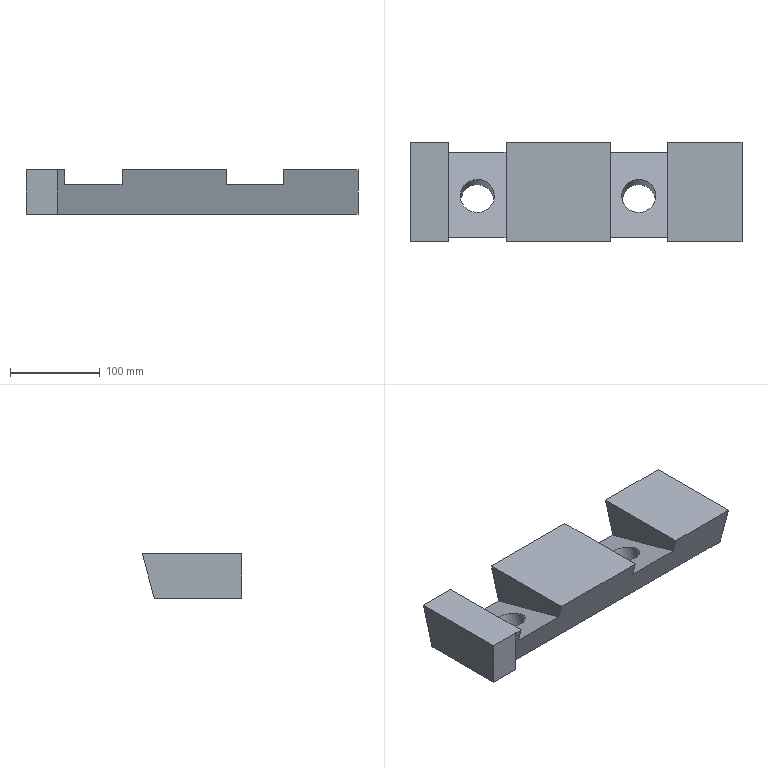Part | SolidWorks | features ICE 3, Extrusion 1, LPattern 1, RevCut 1 | 1 solid | 20 faces | box 370 x 110.795 x 50 mm | volume 1371734 mm3 | plane 16 | cylinder 4 | commonest cylinder face diameters 38 x4
STEP:
#1=CARTESIAN_POINT('',(70.,69.461,-33.943));
#2=VERTEX_POINT('',#1);
#3=CARTESIAN_POINT('',(70.,32.616,-24.071));
#4=VERTEX_POINT('',#3);
#5=CARTESIAN_POINT('',(70.,69.461,-33.943));
#6=CARTESIAN_POINT('',(32.,69.461,-33.943));
#7=CARTESIAN_POINT('',(32.,32.616,-24.071));
#8=CARTESIAN_POINT('',(70.,32.616,-24.071));
#9=(BOUNDED_CURVE()B_SPLINE_CURVE(3,(#5,#6,#7,#8),.UNSPECIFIED.,.F.,.F.)B_SPLINE_CURVE_WITH_KNOTS((4,4),(3.142,6.283),.UNSPECIFIED.)CURVE()GEOMETRIC_REPRESENTATION_ITEM()RATIONAL_B_SPLINE_CURVE((1.,0.3333,0.3333,1.))REPRESENTATION_ITEM(''));
#10=EDGE_CURVE('',#2,#4,#9,.T.);
#11=ORIENTED_EDGE('',*,*,#10,.T.);
#12=CARTESIAN_POINT('',(70.,23.178,-50.));
#13=VERTEX_POINT('',#12);
#14=CARTESIAN_POINT('',(70.,13.311,-77.108));
#15=DIRECTION('',(0.,-0.342,-0.9397));
#16=VECTOR('',#15,1000.);
#17=LINE('',#14,#16);
#18=EDGE_CURVE('',#4,#13,#17,.T.);
#19=ORIENTED_EDGE('',*,*,#18,.T.);
#20=CARTESIAN_POINT('',(70.,63.617,-50.));
#21=VERTEX_POINT('',#20);
#22=CARTESIAN_POINT('',(70.,23.178,-50.));
#23=CARTESIAN_POINT('',(32.,23.178,-50.));
#24=CARTESIAN_POINT('',(32.,63.617,-50.));
#25=CARTESIAN_POINT('',(70.,63.617,-50.));
#26=(BOUNDED_CURVE()B_SPLINE_CURVE(3,(#22,#23,#24,#25),.UNSPECIFIED.,.F.,.F.)B_SPLINE_CURVE_WITH_KNOTS((4,4),(0.,3.142),.UNSPECIFIED.)CURVE()GEOMETRIC_REPRESENTATION_ITEM()RATIONAL_B_SPLINE_CURVE((1.,0.3333,0.3333,1.))REPRESENTATION_ITEM(''));
#27=EDGE_CURVE('',#13,#21,#26,.T.);
#28=ORIENTED_EDGE('',*,*,#27,.T.);
#29=CARTESIAN_POINT('',(70.,49.02,-90.105));
#30=DIRECTION('',(0.,-0.342,-0.9397));
#31=VECTOR('',#30,1000.);
#32=LINE('',#29,#31);
#33=EDGE_CURVE('',#2,#21,#32,.T.);
#34=ORIENTED_EDGE('',*,*,#33,.F.);
#35=EDGE_LOOP('',(#11,#19,#28,#34));
#36=FACE_OUTER_BOUND('',#35,.T.);
#37=CARTESIAN_POINT('',(70.,31.166,-83.607));
#38=DIRECTION('',(0.,-0.342,-0.9397));
#39=DIRECTION('',(0.,0.9397,-0.342));
#40=AXIS2_PLACEMENT_3D('',#37,#38,#39);
#41=CYLINDRICAL_SURFACE('',#40,19.);
#42=ADVANCED_FACE('',(#36),#41,.F.);
#43=CARTESIAN_POINT('',(-110.,69.461,-33.943));
#44=VERTEX_POINT('',#43);
#45=CARTESIAN_POINT('',(-110.,32.616,-24.071));
#46=VERTEX_POINT('',#45);
#47=CARTESIAN_POINT('',(-110.,69.461,-33.943));
#48=CARTESIAN_POINT('',(-148.,69.461,-33.943));
#49=CARTESIAN_POINT('',(-148.,32.616,-24.071));
#50=CARTESIAN_POINT('',(-110.,32.616,-24.071));
#51=(BOUNDED_CURVE()B_SPLINE_CURVE(3,(#47,#48,#49,#50),.UNSPECIFIED.,.F.,.F.)B_SPLINE_CURVE_WITH_KNOTS((4,4),(3.142,6.283),.UNSPECIFIED.)CURVE()GEOMETRIC_REPRESENTATION_ITEM()RATIONAL_B_SPLINE_CURVE((1.,0.3333,0.3333,1.))REPRESENTATION_ITEM(''));
#52=EDGE_CURVE('',#44,#46,#51,.T.);
#53=ORIENTED_EDGE('',*,*,#52,.T.);
#54=CARTESIAN_POINT('',(-110.,23.178,-50.));
#55=VERTEX_POINT('',#54);
#56=CARTESIAN_POINT('',(-110.,13.311,-77.108));
#57=DIRECTION('',(0.,-0.342,-0.9397));
#58=VECTOR('',#57,1000.);
#59=LINE('',#56,#58);
#60=EDGE_CURVE('',#46,#55,#59,.T.);
#61=ORIENTED_EDGE('',*,*,#60,.T.);
#62=CARTESIAN_POINT('',(-110.,63.617,-50.));
#63=VERTEX_POINT('',#62);
#64=CARTESIAN_POINT('',(-110.,23.178,-50.));
#65=CARTESIAN_POINT('',(-148.,23.178,-50.));
#66=CARTESIAN_POINT('',(-148.,63.617,-50.));
#67=CARTESIAN_POINT('',(-110.,63.617,-50.));
#68=(BOUNDED_CURVE()B_SPLINE_CURVE(3,(#64,#65,#66,#67),.UNSPECIFIED.,.F.,.F.)B_SPLINE_CURVE_WITH_KNOTS((4,4),(0.,3.142),.UNSPECIFIED.)CURVE()GEOMETRIC_REPRESENTATION_ITEM()RATIONAL_B_SPLINE_CURVE((1.,0.3333,0.3333,1.))REPRESENTATION_ITEM(''));
#69=EDGE_CURVE('',#55,#63,#68,.T.);
#70=ORIENTED_EDGE('',*,*,#69,.T.);
#71=CARTESIAN_POINT('',(-110.,49.02,-90.105));
#72=DIRECTION('',(0.,-0.342,-0.9397));
#73=VECTOR('',#72,1000.);
#74=LINE('',#71,#73);
#75=EDGE_CURVE('',#44,#63,#74,.T.);
#76=ORIENTED_EDGE('',*,*,#75,.F.);
#77=EDGE_LOOP('',(#53,#61,#70,#76));
#78=FACE_OUTER_BOUND('',#77,.T.);
#79=CARTESIAN_POINT('',(-110.,31.166,-83.607));
#80=DIRECTION('',(0.,-0.342,-0.9397));
#81=DIRECTION('',(0.,0.9397,-0.342));
#82=AXIS2_PLACEMENT_3D('',#79,#80,#81);
#83=CYLINDRICAL_SURFACE('',#82,19.);
#84=ADVANCED_FACE('',(#78),#83,.F.);
#85=CARTESIAN_POINT('',(102.,110.795,0.));
#86=VERTEX_POINT('',#85);
#87=CARTESIAN_POINT('',(102.,0.,0.));
#88=VERTEX_POINT('',#87);
#89=CARTESIAN_POINT('',(102.,110.795,0.));
#90=DIRECTION('',(0.,-1.,0.));
#91=VECTOR('',#90,1000.);
#92=LINE('',#89,#91);
#93=EDGE_CURVE('',#86,#88,#92,.T.);
#94=ORIENTED_EDGE('',*,*,#93,.T.);
#95=CARTESIAN_POINT('',(185.,0.,0.));
#96=VERTEX_POINT('',#95);
#97=CARTESIAN_POINT('',(185.,0.,0.));
#98=DIRECTION('',(-1.,0.,0.));
#99=VECTOR('',#98,1000.);
#100=LINE('',#97,#99);
#101=EDGE_CURVE('',#96,#88,#100,.T.);
#102=ORIENTED_EDGE('',*,*,#101,.F.);
#103=CARTESIAN_POINT('',(185.,110.795,0.));
#104=VERTEX_POINT('',#103);
#105=CARTESIAN_POINT('',(185.,0.,0.));
#106=DIRECTION('',(0.,-1.,0.));
#107=VECTOR('',#106,1000.);
#108=LINE('',#105,#107);
#109=EDGE_CURVE('',#104,#96,#108,.T.);
#110=ORIENTED_EDGE('',*,*,#109,.F.);
#111=CARTESIAN_POINT('',(185.,110.795,0.));
#112=DIRECTION('',(-1.,0.,0.));
#113=VECTOR('',#112,1000.);
#114=LINE('',#111,#113);
#115=EDGE_CURVE('',#104,#86,#114,.T.);
#116=ORIENTED_EDGE('',*,*,#115,.T.);
#117=EDGE_LOOP('',(#94,#102,#110,#116));
#118=FACE_OUTER_BOUND('',#117,.T.);
#119=CARTESIAN_POINT('',(185.,0.,0.));
#120=DIRECTION('',(0.,0.,-1.));
#121=DIRECTION('',(0.,1.,0.));
#122=AXIS2_PLACEMENT_3D('',#119,#120,#121);
#123=PLANE('',#122);
#124=ADVANCED_FACE('',(#118),#123,.F.);
#125=CARTESIAN_POINT('',(38.,0.,0.));
#126=VERTEX_POINT('',#125);
#127=CARTESIAN_POINT('',(-78.,0.,0.));
#128=VERTEX_POINT('',#127);
#129=CARTESIAN_POINT('',(185.,0.,0.));
#130=DIRECTION('',(-1.,0.,0.));
#131=VECTOR('',#130,1000.);
#132=LINE('',#129,#131);
#133=EDGE_CURVE('',#126,#128,#132,.T.);
#134=ORIENTED_EDGE('',*,*,#133,.F.);
#135=CARTESIAN_POINT('',(38.,110.795,0.));
#136=VERTEX_POINT('',#135);
#137=CARTESIAN_POINT('',(38.,110.795,0.));
#138=DIRECTION('',(0.,-1.,0.));
#139=VECTOR('',#138,1000.);
#140=LINE('',#137,#139);
#141=EDGE_CURVE('',#136,#126,#140,.T.);
#142=ORIENTED_EDGE('',*,*,#141,.F.);
#143=CARTESIAN_POINT('',(-78.,110.795,0.));
#144=VERTEX_POINT('',#143);
#145=CARTESIAN_POINT('',(185.,110.795,0.));
#146=DIRECTION('',(-1.,0.,0.));
#147=VECTOR('',#146,1000.);
#148=LINE('',#145,#147);
#149=EDGE_CURVE('',#136,#144,#148,.T.);
#150=ORIENTED_EDGE('',*,*,#149,.T.);
#151=CARTESIAN_POINT('',(-78.,110.795,0.));
#152=DIRECTION('',(0.,-1.,0.));
#153=VECTOR('',#152,1000.);
#154=LINE('',#151,#153);
#155=EDGE_CURVE('',#144,#128,#154,.T.);
#156=ORIENTED_EDGE('',*,*,#155,.T.);
#157=EDGE_LOOP('',(#134,#142,#150,#156));
#158=FACE_OUTER_BOUND('',#157,.T.);
#159=CARTESIAN_POINT('',(185.,0.,0.));
#160=DIRECTION('',(0.,0.,-1.));
#161=DIRECTION('',(0.,1.,0.));
#162=AXIS2_PLACEMENT_3D('',#159,#160,#161);
#163=PLANE('',#162);
#164=ADVANCED_FACE('',(#158),#163,.F.);
#165=CARTESIAN_POINT('',(38.,4.426,-16.517));
#166=VERTEX_POINT('',#165);
#167=CARTESIAN_POINT('',(102.,4.426,-16.517));
#168=VERTEX_POINT('',#167);
#169=CARTESIAN_POINT('',(38.,4.426,-16.517));
#170=DIRECTION('',(1.,0.,0.));
#171=VECTOR('',#170,1000.);
#172=LINE('',#169,#171);
#173=EDGE_CURVE('',#166,#168,#172,.T.);
#174=ORIENTED_EDGE('',*,*,#173,.F.);
#175=CARTESIAN_POINT('',(38.,0.,0.));
#176=DIRECTION('',(0.,0.2588,-0.9659));
#177=VECTOR('',#176,1000.);
#178=LINE('',#175,#177);
#179=EDGE_CURVE('',#126,#166,#178,.T.);
#180=ORIENTED_EDGE('',*,*,#179,.F.);
#181=ORIENTED_EDGE('',*,*,#133,.T.);
#182=CARTESIAN_POINT('',(-78.,4.426,-16.517));
#183=VERTEX_POINT('',#182);
#184=CARTESIAN_POINT('',(-78.,0.,0.));
#185=DIRECTION('',(0.,0.2588,-0.9659));
#186=VECTOR('',#185,1000.);
#187=LINE('',#184,#186);
#188=EDGE_CURVE('',#128,#183,#187,.T.);
#189=ORIENTED_EDGE('',*,*,#188,.T.);
#190=CARTESIAN_POINT('',(-142.,4.426,-16.517));
#191=VERTEX_POINT('',#190);
#192=CARTESIAN_POINT('',(-142.,4.426,-16.517));
#193=DIRECTION('',(1.,0.,0.));
#194=VECTOR('',#193,1000.);
#195=LINE('',#192,#194);
#196=EDGE_CURVE('',#191,#183,#195,.T.);
#197=ORIENTED_EDGE('',*,*,#196,.F.);
#198=CARTESIAN_POINT('',(-142.,0.,0.));
#199=VERTEX_POINT('',#198);
#200=CARTESIAN_POINT('',(-142.,0.,0.));
#201=DIRECTION('',(0.,0.2588,-0.9659));
#202=VECTOR('',#201,1000.);
#203=LINE('',#200,#202);
#204=EDGE_CURVE('',#199,#191,#203,.T.);
#205=ORIENTED_EDGE('',*,*,#204,.F.);
#206=CARTESIAN_POINT('',(-150.,0.,0.));
#207=VERTEX_POINT('',#206);
#208=CARTESIAN_POINT('',(185.,0.,0.));
#209=DIRECTION('',(-1.,0.,0.));
#210=VECTOR('',#209,1000.);
#211=LINE('',#208,#210);
#212=EDGE_CURVE('',#199,#207,#211,.T.);
#213=ORIENTED_EDGE('',*,*,#212,.T.);
#214=CARTESIAN_POINT('',(-150.,13.397,-50.));
#215=VERTEX_POINT('',#214);
#216=CARTESIAN_POINT('',(-150.,13.397,-50.));
#217=DIRECTION('',(0.,0.2588,-0.9659));
#218=VECTOR('',#217,1000.);
#219=LINE('',#216,#218);
#220=EDGE_CURVE('',#207,#215,#219,.T.);
#221=ORIENTED_EDGE('',*,*,#220,.T.);
#222=CARTESIAN_POINT('',(185.,13.397,-50.));
#223=VERTEX_POINT('',#222);
#224=CARTESIAN_POINT('',(185.,13.397,-50.));
#225=DIRECTION('',(-1.,0.,0.));
#226=VECTOR('',#225,1000.);
#227=LINE('',#224,#226);
#228=EDGE_CURVE('',#223,#215,#227,.T.);
#229=ORIENTED_EDGE('',*,*,#228,.F.);
#230=CARTESIAN_POINT('',(185.,13.397,-50.));
#231=DIRECTION('',(0.,0.2588,-0.9659));
#232=VECTOR('',#231,1000.);
#233=LINE('',#230,#232);
#234=EDGE_CURVE('',#96,#223,#233,.T.);
#235=ORIENTED_EDGE('',*,*,#234,.F.);
#236=ORIENTED_EDGE('',*,*,#101,.T.);
#237=CARTESIAN_POINT('',(102.,0.,0.));
#238=DIRECTION('',(0.,0.2588,-0.9659));
#239=VECTOR('',#238,1000.);
#240=LINE('',#237,#239);
#241=EDGE_CURVE('',#88,#168,#240,.T.);
#242=ORIENTED_EDGE('',*,*,#241,.T.);
#243=EDGE_LOOP('',(#174,#180,#181,#189,#197,#205,#213,#221,#229,#235,#236,#242));
#244=FACE_OUTER_BOUND('',#243,.T.);
#245=CARTESIAN_POINT('',(185.,13.397,-50.));
#246=DIRECTION('',(0.,0.9659,0.2588));
#247=DIRECTION('',(0.,-0.2588,0.9659));
#248=AXIS2_PLACEMENT_3D('',#245,#246,#247);
#249=PLANE('',#248);
#250=ADVANCED_FACE('',(#244),#249,.F.);
#251=CARTESIAN_POINT('',(70.,63.617,-50.));
#252=CARTESIAN_POINT('',(108.,63.617,-50.));
#253=CARTESIAN_POINT('',(108.,23.178,-50.));
#254=CARTESIAN_POINT('',(70.,23.178,-50.));
#255=(BOUNDED_CURVE()B_SPLINE_CURVE(3,(#251,#252,#253,#254),.UNSPECIFIED.,.F.,.T.)B_SPLINE_CURVE_WITH_KNOTS((4,4),(3.142,6.283),.UNSPECIFIED.)CURVE()GEOMETRIC_REPRESENTATION_ITEM()RATIONAL_B_SPLINE_CURVE((1.,0.3333,0.3333,1.))REPRESENTATION_ITEM(''));
#256=EDGE_CURVE('',#21,#13,#255,.T.);
#257=ORIENTED_EDGE('',*,*,#256,.F.);
#258=ORIENTED_EDGE('',*,*,#27,.F.);
#259=EDGE_LOOP('',(#257,#258));
#260=FACE_BOUND('',#259,.T.);
#261=CARTESIAN_POINT('',(-110.,63.617,-50.));
#262=CARTESIAN_POINT('',(-72.,63.617,-50.));
#263=CARTESIAN_POINT('',(-72.,23.178,-50.));
#264=CARTESIAN_POINT('',(-110.,23.178,-50.));
#265=(BOUNDED_CURVE()B_SPLINE_CURVE(3,(#261,#262,#263,#264),.UNSPECIFIED.,.F.,.T.)B_SPLINE_CURVE_WITH_KNOTS((4,4),(3.142,6.283),.UNSPECIFIED.)CURVE()GEOMETRIC_REPRESENTATION_ITEM()RATIONAL_B_SPLINE_CURVE((1.,0.3333,0.3333,1.))REPRESENTATION_ITEM(''));
#266=EDGE_CURVE('',#63,#55,#265,.T.);
#267=ORIENTED_EDGE('',*,*,#266,.F.);
#268=ORIENTED_EDGE('',*,*,#69,.F.);
#269=EDGE_LOOP('',(#267,#268));
#270=FACE_BOUND('',#269,.T.);
#271=CARTESIAN_POINT('',(-185.,0.,-50.));
#272=VERTEX_POINT('',#271);
#273=CARTESIAN_POINT('',(-185.,97.397,-50.));
#274=VERTEX_POINT('',#273);
#275=CARTESIAN_POINT('',(-185.,97.397,-50.));
#276=DIRECTION('',(0.,1.,0.));
#277=VECTOR('',#276,1000.);
#278=LINE('',#275,#277);
#279=EDGE_CURVE('',#272,#274,#278,.T.);
#280=ORIENTED_EDGE('',*,*,#279,.T.);
#281=CARTESIAN_POINT('',(185.,97.397,-50.));
#282=VERTEX_POINT('',#281);
#283=CARTESIAN_POINT('',(185.,97.397,-50.));
#284=DIRECTION('',(-1.,0.,0.));
#285=VECTOR('',#284,1000.);
#286=LINE('',#283,#285);
#287=EDGE_CURVE('',#282,#274,#286,.T.);
#288=ORIENTED_EDGE('',*,*,#287,.F.);
#289=CARTESIAN_POINT('',(185.,97.397,-50.));
#290=DIRECTION('',(0.,1.,0.));
#291=VECTOR('',#290,1000.);
#292=LINE('',#289,#291);
#293=EDGE_CURVE('',#223,#282,#292,.T.);
#294=ORIENTED_EDGE('',*,*,#293,.F.);
#295=ORIENTED_EDGE('',*,*,#228,.T.);
#296=CARTESIAN_POINT('',(-150.,0.,-50.));
#297=VERTEX_POINT('',#296);
#298=CARTESIAN_POINT('',(-150.,0.,-50.));
#299=DIRECTION('',(0.,-1.,0.));
#300=VECTOR('',#299,1000.);
#301=LINE('',#298,#300);
#302=EDGE_CURVE('',#215,#297,#301,.T.);
#303=ORIENTED_EDGE('',*,*,#302,.T.);
#304=CARTESIAN_POINT('',(-150.,0.,-50.));
#305=DIRECTION('',(-1.,0.,0.));
#306=VECTOR('',#305,1000.);
#307=LINE('',#304,#306);
#308=EDGE_CURVE('',#297,#272,#307,.T.);
#309=ORIENTED_EDGE('',*,*,#308,.T.);
#310=EDGE_LOOP('',(#280,#288,#294,#295,#303,#309));
#311=FACE_OUTER_BOUND('',#310,.T.);
#312=CARTESIAN_POINT('',(185.,97.397,-50.));
#313=DIRECTION('',(0.,0.,1.));
#314=DIRECTION('',(0.,-1.,0.));
#315=AXIS2_PLACEMENT_3D('',#312,#313,#314);
#316=PLANE('',#315);
#317=ADVANCED_FACE('',(#260,#270,#311),#316,.F.);
#318=ORIENTED_EDGE('',*,*,#149,.F.);
#319=CARTESIAN_POINT('',(38.,99.54,-42.003));
#320=VERTEX_POINT('',#319);
#321=CARTESIAN_POINT('',(38.,99.54,-42.003));
#322=DIRECTION('',(0.,0.2588,0.9659));
#323=VECTOR('',#322,1000.);
#324=LINE('',#321,#323);
#325=EDGE_CURVE('',#320,#136,#324,.T.);
#326=ORIENTED_EDGE('',*,*,#325,.F.);
#327=CARTESIAN_POINT('',(102.,99.54,-42.003));
#328=VERTEX_POINT('',#327);
#329=CARTESIAN_POINT('',(38.,99.54,-42.003));
#330=DIRECTION('',(1.,0.,0.));
#331=VECTOR('',#330,1000.);
#332=LINE('',#329,#331);
#333=EDGE_CURVE('',#320,#328,#332,.T.);
#334=ORIENTED_EDGE('',*,*,#333,.T.);
#335=CARTESIAN_POINT('',(102.,99.54,-42.003));
#336=DIRECTION('',(0.,0.2588,0.9659));
#337=VECTOR('',#336,1000.);
#338=LINE('',#335,#337);
#339=EDGE_CURVE('',#328,#86,#338,.T.);
#340=ORIENTED_EDGE('',*,*,#339,.T.);
#341=ORIENTED_EDGE('',*,*,#115,.F.);
#342=CARTESIAN_POINT('',(185.,110.795,0.));
#343=DIRECTION('',(0.,0.2588,0.9659));
#344=VECTOR('',#343,1000.);
#345=LINE('',#342,#344);
#346=EDGE_CURVE('',#282,#104,#345,.T.);
#347=ORIENTED_EDGE('',*,*,#346,.F.);
#348=ORIENTED_EDGE('',*,*,#287,.T.);
#349=CARTESIAN_POINT('',(-185.,110.795,0.));
#350=VERTEX_POINT('',#349);
#351=CARTESIAN_POINT('',(-185.,110.795,0.));
#352=DIRECTION('',(0.,0.2588,0.9659));
#353=VECTOR('',#352,1000.);
#354=LINE('',#351,#353);
#355=EDGE_CURVE('',#274,#350,#354,.T.);
#356=ORIENTED_EDGE('',*,*,#355,.T.);
#357=CARTESIAN_POINT('',(-142.,110.795,0.));
#358=VERTEX_POINT('',#357);
#359=CARTESIAN_POINT('',(185.,110.795,0.));
#360=DIRECTION('',(-1.,0.,0.));
#361=VECTOR('',#360,1000.);
#362=LINE('',#359,#361);
#363=EDGE_CURVE('',#358,#350,#362,.T.);
#364=ORIENTED_EDGE('',*,*,#363,.F.);
#365=CARTESIAN_POINT('',(-142.,99.54,-42.003));
#366=VERTEX_POINT('',#365);
#367=CARTESIAN_POINT('',(-142.,99.54,-42.003));
#368=DIRECTION('',(0.,0.2588,0.9659));
#369=VECTOR('',#368,1000.);
#370=LINE('',#367,#369);
#371=EDGE_CURVE('',#366,#358,#370,.T.);
#372=ORIENTED_EDGE('',*,*,#371,.F.);
#373=CARTESIAN_POINT('',(-78.,99.54,-42.003));
#374=VERTEX_POINT('',#373);
#375=CARTESIAN_POINT('',(-142.,99.54,-42.003));
#376=DIRECTION('',(1.,0.,0.));
#377=VECTOR('',#376,1000.);
#378=LINE('',#375,#377);
#379=EDGE_CURVE('',#366,#374,#378,.T.);
#380=ORIENTED_EDGE('',*,*,#379,.T.);
#381=CARTESIAN_POINT('',(-78.,99.54,-42.003));
#382=DIRECTION('',(0.,0.2588,0.9659));
#383=VECTOR('',#382,1000.);
#384=LINE('',#381,#383);
#385=EDGE_CURVE('',#374,#144,#384,.T.);
#386=ORIENTED_EDGE('',*,*,#385,.T.);
#387=EDGE_LOOP('',(#318,#326,#334,#340,#341,#347,#348,#356,#364,#372,#380,#386));
#388=FACE_OUTER_BOUND('',#387,.T.);
#389=CARTESIAN_POINT('',(185.,110.795,0.));
#390=DIRECTION('',(0.,-0.9659,0.2588));
#391=DIRECTION('',(0.,-0.2588,-0.9659));
#392=AXIS2_PLACEMENT_3D('',#389,#390,#391);
#393=PLANE('',#392);
#394=ADVANCED_FACE('',(#388),#393,.F.);
#395=ORIENTED_EDGE('',*,*,#212,.F.);
#396=CARTESIAN_POINT('',(-142.,110.795,0.));
#397=DIRECTION('',(0.,-1.,0.));
#398=VECTOR('',#397,1000.);
#399=LINE('',#396,#398);
#400=EDGE_CURVE('',#358,#199,#399,.T.);
#401=ORIENTED_EDGE('',*,*,#400,.F.);
#402=ORIENTED_EDGE('',*,*,#363,.T.);
#403=CARTESIAN_POINT('',(-185.,0.,0.));
#404=VERTEX_POINT('',#403);
#405=CARTESIAN_POINT('',(-185.,0.,0.));
#406=DIRECTION('',(0.,-1.,0.));
#407=VECTOR('',#406,1000.);
#408=LINE('',#405,#407);
#409=EDGE_CURVE('',#350,#404,#408,.T.);
#410=ORIENTED_EDGE('',*,*,#409,.T.);
#411=CARTESIAN_POINT('',(-150.,0.,0.));
#412=DIRECTION('',(-1.,0.,0.));
#413=VECTOR('',#412,1000.);
#414=LINE('',#411,#413);
#415=EDGE_CURVE('',#207,#404,#414,.T.);
#416=ORIENTED_EDGE('',*,*,#415,.F.);
#417=EDGE_LOOP('',(#395,#401,#402,#410,#416));
#418=FACE_OUTER_BOUND('',#417,.T.);
#419=CARTESIAN_POINT('',(185.,0.,0.));
#420=DIRECTION('',(0.,0.,-1.));
#421=DIRECTION('',(0.,1.,0.));
#422=AXIS2_PLACEMENT_3D('',#419,#420,#421);
#423=PLANE('',#422);
#424=ADVANCED_FACE('',(#418),#423,.F.);
#425=ORIENTED_EDGE('',*,*,#234,.T.);
#426=ORIENTED_EDGE('',*,*,#293,.T.);
#427=ORIENTED_EDGE('',*,*,#346,.T.);
#428=ORIENTED_EDGE('',*,*,#109,.T.);
#429=EDGE_LOOP('',(#425,#426,#427,#428));
#430=FACE_OUTER_BOUND('',#429,.T.);
#431=CARTESIAN_POINT('',(185.,0.,0.));
#432=DIRECTION('',(-1.,0.,0.));
#433=DIRECTION('',(0.,0.,1.));
#434=AXIS2_PLACEMENT_3D('',#431,#432,#433);
#435=PLANE('',#434);
#436=ADVANCED_FACE('',(#430),#435,.F.);
#437=ORIENTED_EDGE('',*,*,#279,.F.);
#438=CARTESIAN_POINT('',(-185.,0.,0.));
#439=DIRECTION('',(0.,0.,1.));
#440=VECTOR('',#439,1000.);
#441=LINE('',#438,#440);
#442=EDGE_CURVE('',#272,#404,#441,.T.);
#443=ORIENTED_EDGE('',*,*,#442,.T.);
#444=ORIENTED_EDGE('',*,*,#409,.F.);
#445=ORIENTED_EDGE('',*,*,#355,.F.);
#446=EDGE_LOOP('',(#437,#443,#444,#445));
#447=FACE_OUTER_BOUND('',#446,.T.);
#448=CARTESIAN_POINT('',(-185.,0.,0.));
#449=DIRECTION('',(-1.,0.,0.));
#450=DIRECTION('',(0.,0.,1.));
#451=AXIS2_PLACEMENT_3D('',#448,#449,#450);
#452=PLANE('',#451);
#453=ADVANCED_FACE('',(#447),#452,.T.);
#454=ORIENTED_EDGE('',*,*,#442,.F.);
#455=ORIENTED_EDGE('',*,*,#308,.F.);
#456=CARTESIAN_POINT('',(-150.,0.,0.));
#457=DIRECTION('',(0.,0.,1.));
#458=VECTOR('',#457,1000.);
#459=LINE('',#456,#458);
#460=EDGE_CURVE('',#297,#207,#459,.T.);
#461=ORIENTED_EDGE('',*,*,#460,.T.);
#462=ORIENTED_EDGE('',*,*,#415,.T.);
#463=EDGE_LOOP('',(#454,#455,#461,#462));
#464=FACE_OUTER_BOUND('',#463,.T.);
#465=CARTESIAN_POINT('',(-150.,0.,0.));
#466=DIRECTION('',(0.,-1.,0.));
#467=DIRECTION('',(0.,0.,-1.));
#468=AXIS2_PLACEMENT_3D('',#465,#466,#467);
#469=PLANE('',#468);
#470=ADVANCED_FACE('',(#464),#469,.T.);
#471=ORIENTED_EDGE('',*,*,#220,.F.);
#472=ORIENTED_EDGE('',*,*,#460,.F.);
#473=ORIENTED_EDGE('',*,*,#302,.F.);
#474=EDGE_LOOP('',(#471,#472,#473));
#475=FACE_OUTER_BOUND('',#474,.T.);
#476=CARTESIAN_POINT('',(-150.,0.,0.));
#477=DIRECTION('',(-1.,0.,0.));
#478=DIRECTION('',(0.,0.,1.));
#479=AXIS2_PLACEMENT_3D('',#476,#477,#478);
#480=PLANE('',#479);
#481=ADVANCED_FACE('',(#475),#480,.F.);
#482=ORIENTED_EDGE('',*,*,#52,.F.);
#483=CARTESIAN_POINT('',(-110.,32.616,-24.071));
#484=CARTESIAN_POINT('',(-72.,32.616,-24.071));
#485=CARTESIAN_POINT('',(-72.,69.461,-33.943));
#486=CARTESIAN_POINT('',(-110.,69.461,-33.943));
#487=(BOUNDED_CURVE()B_SPLINE_CURVE(3,(#483,#484,#485,#486),.UNSPECIFIED.,.F.,.F.)B_SPLINE_CURVE_WITH_KNOTS((4,4),(0.,3.142),.UNSPECIFIED.)CURVE()GEOMETRIC_REPRESENTATION_ITEM()RATIONAL_B_SPLINE_CURVE((1.,0.3333,0.3333,1.))REPRESENTATION_ITEM(''));
#488=EDGE_CURVE('',#46,#44,#487,.T.);
#489=ORIENTED_EDGE('',*,*,#488,.F.);
#490=EDGE_LOOP('',(#482,#489));
#491=FACE_BOUND('',#490,.T.);
#492=CARTESIAN_POINT('',(-78.,4.426,-16.517));
#493=DIRECTION('',(0.,0.9659,-0.2588));
#494=VECTOR('',#493,1000.);
#495=LINE('',#492,#494);
#496=EDGE_CURVE('',#183,#374,#495,.T.);
#497=ORIENTED_EDGE('',*,*,#496,.T.);
#498=ORIENTED_EDGE('',*,*,#379,.F.);
#499=CARTESIAN_POINT('',(-142.,4.426,-16.517));
#500=DIRECTION('',(0.,0.9659,-0.2588));
#501=VECTOR('',#500,1000.);
#502=LINE('',#499,#501);
#503=EDGE_CURVE('',#191,#366,#502,.T.);
#504=ORIENTED_EDGE('',*,*,#503,.F.);
#505=ORIENTED_EDGE('',*,*,#196,.T.);
#506=EDGE_LOOP('',(#497,#498,#504,#505));
#507=FACE_OUTER_BOUND('',#506,.T.);
#508=CARTESIAN_POINT('',(-142.,4.426,-16.517));
#509=DIRECTION('',(0.,-0.2588,-0.9659));
#510=DIRECTION('',(0.,0.9659,-0.2588));
#511=AXIS2_PLACEMENT_3D('',#508,#509,#510);
#512=PLANE('',#511);
#513=ADVANCED_FACE('',(#491,#507),#512,.F.);
#514=ORIENTED_EDGE('',*,*,#204,.T.);
#515=ORIENTED_EDGE('',*,*,#503,.T.);
#516=ORIENTED_EDGE('',*,*,#371,.T.);
#517=ORIENTED_EDGE('',*,*,#400,.T.);
#518=EDGE_LOOP('',(#514,#515,#516,#517));
#519=FACE_OUTER_BOUND('',#518,.T.);
#520=CARTESIAN_POINT('',(-142.,0.,0.));
#521=DIRECTION('',(-1.,0.,0.));
#522=DIRECTION('',(0.,0.,1.));
#523=AXIS2_PLACEMENT_3D('',#520,#521,#522);
#524=PLANE('',#523);
#525=ADVANCED_FACE('',(#519),#524,.F.);
#526=ORIENTED_EDGE('',*,*,#188,.F.);
#527=ORIENTED_EDGE('',*,*,#155,.F.);
#528=ORIENTED_EDGE('',*,*,#385,.F.);
#529=ORIENTED_EDGE('',*,*,#496,.F.);
#530=EDGE_LOOP('',(#526,#527,#528,#529));
#531=FACE_OUTER_BOUND('',#530,.T.);
#532=CARTESIAN_POINT('',(-78.,0.,0.));
#533=DIRECTION('',(-1.,0.,0.));
#534=DIRECTION('',(0.,0.,1.));
#535=AXIS2_PLACEMENT_3D('',#532,#533,#534);
#536=PLANE('',#535);
#537=ADVANCED_FACE('',(#531),#536,.T.);
#538=ORIENTED_EDGE('',*,*,#10,.F.);
#539=CARTESIAN_POINT('',(70.,32.616,-24.071));
#540=CARTESIAN_POINT('',(108.,32.616,-24.071));
#541=CARTESIAN_POINT('',(108.,69.461,-33.943));
#542=CARTESIAN_POINT('',(70.,69.461,-33.943));
#543=(BOUNDED_CURVE()B_SPLINE_CURVE(3,(#539,#540,#541,#542),.UNSPECIFIED.,.F.,.F.)B_SPLINE_CURVE_WITH_KNOTS((4,4),(0.,3.142),.UNSPECIFIED.)CURVE()GEOMETRIC_REPRESENTATION_ITEM()RATIONAL_B_SPLINE_CURVE((1.,0.3333,0.3333,1.))REPRESENTATION_ITEM(''));
#544=EDGE_CURVE('',#4,#2,#543,.T.);
#545=ORIENTED_EDGE('',*,*,#544,.F.);
#546=EDGE_LOOP('',(#538,#545));
#547=FACE_BOUND('',#546,.T.);
#548=CARTESIAN_POINT('',(102.,4.426,-16.517));
#549=DIRECTION('',(0.,0.9659,-0.2588));
#550=VECTOR('',#549,1000.);
#551=LINE('',#548,#550);
#552=EDGE_CURVE('',#168,#328,#551,.T.);
#553=ORIENTED_EDGE('',*,*,#552,.T.);
#554=ORIENTED_EDGE('',*,*,#333,.F.);
#555=CARTESIAN_POINT('',(38.,4.426,-16.517));
#556=DIRECTION('',(0.,0.9659,-0.2588));
#557=VECTOR('',#556,1000.);
#558=LINE('',#555,#557);
#559=EDGE_CURVE('',#166,#320,#558,.T.);
#560=ORIENTED_EDGE('',*,*,#559,.F.);
#561=ORIENTED_EDGE('',*,*,#173,.T.);
#562=EDGE_LOOP('',(#553,#554,#560,#561));
#563=FACE_OUTER_BOUND('',#562,.T.);
#564=CARTESIAN_POINT('',(38.,4.426,-16.517));
#565=DIRECTION('',(0.,-0.2588,-0.9659));
#566=DIRECTION('',(0.,0.9659,-0.2588));
#567=AXIS2_PLACEMENT_3D('',#564,#565,#566);
#568=PLANE('',#567);
#569=ADVANCED_FACE('',(#547,#563),#568,.F.);
#570=ORIENTED_EDGE('',*,*,#179,.T.);
#571=ORIENTED_EDGE('',*,*,#559,.T.);
#572=ORIENTED_EDGE('',*,*,#325,.T.);
#573=ORIENTED_EDGE('',*,*,#141,.T.);
#574=EDGE_LOOP('',(#570,#571,#572,#573));
#575=FACE_OUTER_BOUND('',#574,.T.);
#576=CARTESIAN_POINT('',(38.,0.,0.));
#577=DIRECTION('',(-1.,0.,0.));
#578=DIRECTION('',(0.,0.,1.));
#579=AXIS2_PLACEMENT_3D('',#576,#577,#578);
#580=PLANE('',#579);
#581=ADVANCED_FACE('',(#575),#580,.F.);
#582=ORIENTED_EDGE('',*,*,#241,.F.);
#583=ORIENTED_EDGE('',*,*,#93,.F.);
#584=ORIENTED_EDGE('',*,*,#339,.F.);
#585=ORIENTED_EDGE('',*,*,#552,.F.);
#586=EDGE_LOOP('',(#582,#583,#584,#585));
#587=FACE_OUTER_BOUND('',#586,.T.);
#588=CARTESIAN_POINT('',(102.,0.,0.));
#589=DIRECTION('',(-1.,0.,0.));
#590=DIRECTION('',(0.,0.,1.));
#591=AXIS2_PLACEMENT_3D('',#588,#589,#590);
#592=PLANE('',#591);
#593=ADVANCED_FACE('',(#587),#592,.T.);
#594=ORIENTED_EDGE('',*,*,#60,.F.);
#595=ORIENTED_EDGE('',*,*,#488,.T.);
#596=ORIENTED_EDGE('',*,*,#75,.T.);
#597=ORIENTED_EDGE('',*,*,#266,.T.);
#598=EDGE_LOOP('',(#594,#595,#596,#597));
#599=FACE_OUTER_BOUND('',#598,.T.);
#600=CARTESIAN_POINT('',(-110.,31.166,-83.607));
#601=DIRECTION('',(0.,-0.342,-0.9397));
#602=DIRECTION('',(0.,0.9397,-0.342));
#603=AXIS2_PLACEMENT_3D('',#600,#601,#602);
#604=CYLINDRICAL_SURFACE('',#603,19.);
#605=ADVANCED_FACE('',(#599),#604,.F.);
#606=ORIENTED_EDGE('',*,*,#18,.F.);
#607=ORIENTED_EDGE('',*,*,#544,.T.);
#608=ORIENTED_EDGE('',*,*,#33,.T.);
#609=ORIENTED_EDGE('',*,*,#256,.T.);
#610=EDGE_LOOP('',(#606,#607,#608,#609));
#611=FACE_OUTER_BOUND('',#610,.T.);
#612=CARTESIAN_POINT('',(70.,31.166,-83.607));
#613=DIRECTION('',(0.,-0.342,-0.9397));
#614=DIRECTION('',(0.,0.9397,-0.342));
#615=AXIS2_PLACEMENT_3D('',#612,#613,#614);
#616=CYLINDRICAL_SURFACE('',#615,19.);
#617=ADVANCED_FACE('',(#611),#616,.F.);
#618=CLOSED_SHELL('',(#42,#84,#124,#164,#250,#317,#394,#424,#436,#453,#470,#481,#513,#525,#537,#569,#581,#593,#605,#617));
#619=MANIFOLD_SOLID_BREP('',#618);
#620=CARTESIAN_POINT('',(0.,0.,0.));
#621=DIRECTION('',(0.,0.,1.));
#622=DIRECTION('',(1.,0.,0.));
#623=AXIS2_PLACEMENT_3D('',#620,#621,#622);
#624=(LENGTH_UNIT()NAMED_UNIT(*)SI_UNIT(.MILLI.,.METRE.));
#625=UNCERTAINTY_MEASURE_WITH_UNIT(LENGTH_MEASURE(0.00001),#624,'','');
#626=(NAMED_UNIT(*)PLANE_ANGLE_UNIT()SI_UNIT($,.RADIAN.));
#627=(NAMED_UNIT(*)SI_UNIT($,.STERADIAN.)SOLID_ANGLE_UNIT());
#628=(GEOMETRIC_REPRESENTATION_CONTEXT(3)GLOBAL_UNCERTAINTY_ASSIGNED_CONTEXT((#625))GLOBAL_UNIT_ASSIGNED_CONTEXT((#624,#626,#627))REPRESENTATION_CONTEXT('',''));
#629=ADVANCED_BREP_SHAPE_REPRESENTATION('',(#619,#623),#628);